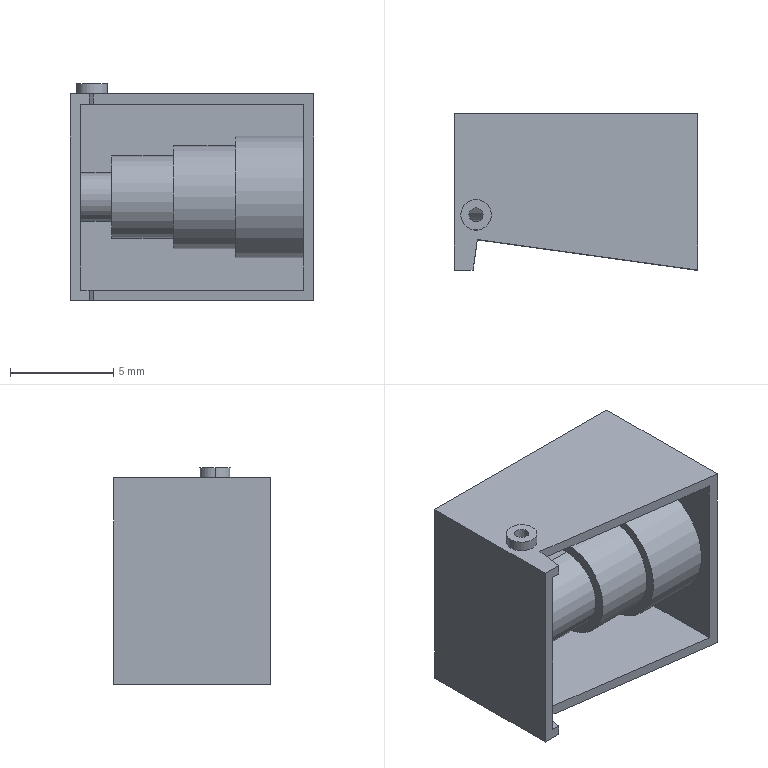Part | SolidWorks | features ICE 8, Extrusion 1, Shell 1 | 1 solid | 35 faces | box 11.794 x 7.578 x 10.5 mm | volume 389.974 mm3 | plane 19 | cylinder 16 | commonest cylinder face diameters 0.684 x4 1.479 x2 1.676 x2 2.353 x2 4 x2 5 x2
STEP:
#1=CARTESIAN_POINT('',(-33.114,-4.039,-2.056));
#2=VERTEX_POINT('',#1);
#3=CARTESIAN_POINT('',(-33.114,-4.039,-7.944));
#4=VERTEX_POINT('',#3);
#5=CARTESIAN_POINT('',(-33.114,-4.039,-5.));
#6=DIRECTION('',(-1.,0.,0.));
#7=DIRECTION('',(0.,0.,-1.));
#8=AXIS2_PLACEMENT_3D('',#5,#6,#7);
#9=CIRCLE('',#8,2.944);
#10=EDGE_CURVE('',#2,#4,#9,.T.);
#11=ORIENTED_EDGE('',*,*,#10,.T.);
#12=CARTESIAN_POINT('',(-36.407,-4.039,-7.944));
#13=VERTEX_POINT('',#12);
#14=CARTESIAN_POINT('',(-24.786,-4.039,-7.944));
#15=DIRECTION('',(-1.,0.,0.));
#16=VECTOR('',#15,1000.);
#17=LINE('',#14,#16);
#18=EDGE_CURVE('',#4,#13,#17,.T.);
#19=ORIENTED_EDGE('',*,*,#18,.T.);
#20=CARTESIAN_POINT('',(-36.407,-4.039,-2.056));
#21=VERTEX_POINT('',#20);
#22=CARTESIAN_POINT('',(-36.407,-4.039,-5.));
#23=DIRECTION('',(1.,0.,0.));
#24=DIRECTION('',(0.,0.,-1.));
#25=AXIS2_PLACEMENT_3D('',#22,#23,#24);
#26=CIRCLE('',#25,2.944);
#27=EDGE_CURVE('',#13,#21,#26,.T.);
#28=ORIENTED_EDGE('',*,*,#27,.T.);
#29=CARTESIAN_POINT('',(-24.786,-4.039,-2.056));
#30=DIRECTION('',(-1.,0.,0.));
#31=VECTOR('',#30,1000.);
#32=LINE('',#29,#31);
#33=EDGE_CURVE('',#2,#21,#32,.T.);
#34=ORIENTED_EDGE('',*,*,#33,.F.);
#35=EDGE_LOOP('',(#11,#19,#28,#34));
#36=FACE_OUTER_BOUND('',#35,.T.);
#37=CARTESIAN_POINT('',(-24.786,-4.039,-5.));
#38=DIRECTION('',(-1.,0.,0.));
#39=DIRECTION('',(0.,0.,1.));
#40=AXIS2_PLACEMENT_3D('',#37,#38,#39);
#41=CYLINDRICAL_SURFACE('',#40,2.944);
#42=ADVANCED_FACE('',(#36),#41,.T.);
#43=CARTESIAN_POINT('',(-36.407,-4.039,-7.5));
#44=VERTEX_POINT('',#43);
#45=CARTESIAN_POINT('',(-36.407,-4.039,-2.5));
#46=VERTEX_POINT('',#45);
#47=CARTESIAN_POINT('',(-36.407,-4.039,-5.));
#48=DIRECTION('',(1.,0.,0.));
#49=DIRECTION('',(0.,0.,-1.));
#50=AXIS2_PLACEMENT_3D('',#47,#48,#49);
#51=CIRCLE('',#50,2.5);
#52=EDGE_CURVE('',#44,#46,#51,.T.);
#53=ORIENTED_EDGE('',*,*,#52,.F.);
#54=CARTESIAN_POINT('',(-39.407,-4.039,-7.5));
#55=VERTEX_POINT('',#54);
#56=CARTESIAN_POINT('',(-36.407,-4.039,-7.5));
#57=DIRECTION('',(-1.,0.,0.));
#58=VECTOR('',#57,1000.);
#59=LINE('',#56,#58);
#60=EDGE_CURVE('',#44,#55,#59,.T.);
#61=ORIENTED_EDGE('',*,*,#60,.T.);
#62=CARTESIAN_POINT('',(-39.407,-4.039,-2.5));
#63=VERTEX_POINT('',#62);
#64=CARTESIAN_POINT('',(-39.407,-4.039,-5.));
#65=DIRECTION('',(1.,0.,0.));
#66=DIRECTION('',(0.,0.,-1.));
#67=AXIS2_PLACEMENT_3D('',#64,#65,#66);
#68=CIRCLE('',#67,2.5);
#69=EDGE_CURVE('',#55,#63,#68,.T.);
#70=ORIENTED_EDGE('',*,*,#69,.T.);
#71=CARTESIAN_POINT('',(-36.407,-4.039,-2.5));
#72=DIRECTION('',(-1.,0.,0.));
#73=VECTOR('',#72,1000.);
#74=LINE('',#71,#73);
#75=EDGE_CURVE('',#46,#63,#74,.T.);
#76=ORIENTED_EDGE('',*,*,#75,.F.);
#77=EDGE_LOOP('',(#53,#61,#70,#76));
#78=FACE_OUTER_BOUND('',#77,.T.);
#79=CARTESIAN_POINT('',(-36.407,-4.039,-5.));
#80=DIRECTION('',(-1.,0.,0.));
#81=DIRECTION('',(0.,0.,1.));
#82=AXIS2_PLACEMENT_3D('',#79,#80,#81);
#83=CYLINDRICAL_SURFACE('',#82,2.5);
#84=ADVANCED_FACE('',(#78),#83,.T.);
#85=CARTESIAN_POINT('',(-39.407,-4.039,-7.));
#86=VERTEX_POINT('',#85);
#87=CARTESIAN_POINT('',(-39.407,-4.039,-3.));
#88=VERTEX_POINT('',#87);
#89=CARTESIAN_POINT('',(-39.407,-4.039,-5.));
#90=DIRECTION('',(1.,0.,0.));
#91=DIRECTION('',(0.,0.,-1.));
#92=AXIS2_PLACEMENT_3D('',#89,#90,#91);
#93=CIRCLE('',#92,2.);
#94=EDGE_CURVE('',#86,#88,#93,.T.);
#95=ORIENTED_EDGE('',*,*,#94,.F.);
#96=CARTESIAN_POINT('',(-42.407,-4.039,-7.));
#97=VERTEX_POINT('',#96);
#98=CARTESIAN_POINT('',(-39.407,-4.039,-7.));
#99=DIRECTION('',(-1.,0.,0.));
#100=VECTOR('',#99,1000.);
#101=LINE('',#98,#100);
#102=EDGE_CURVE('',#86,#97,#101,.T.);
#103=ORIENTED_EDGE('',*,*,#102,.T.);
#104=CARTESIAN_POINT('',(-42.407,-4.039,-3.));
#105=VERTEX_POINT('',#104);
#106=CARTESIAN_POINT('',(-42.407,-4.039,-5.));
#107=DIRECTION('',(1.,0.,0.));
#108=DIRECTION('',(0.,0.,-1.));
#109=AXIS2_PLACEMENT_3D('',#106,#107,#108);
#110=CIRCLE('',#109,2.);
#111=EDGE_CURVE('',#97,#105,#110,.T.);
#112=ORIENTED_EDGE('',*,*,#111,.T.);
#113=CARTESIAN_POINT('',(-39.407,-4.039,-3.));
#114=DIRECTION('',(-1.,0.,0.));
#115=VECTOR('',#114,1000.);
#116=LINE('',#113,#115);
#117=EDGE_CURVE('',#88,#105,#116,.T.);
#118=ORIENTED_EDGE('',*,*,#117,.F.);
#119=EDGE_LOOP('',(#95,#103,#112,#118));
#120=FACE_OUTER_BOUND('',#119,.T.);
#121=CARTESIAN_POINT('',(-39.407,-4.039,-5.));
#122=DIRECTION('',(-1.,0.,0.));
#123=DIRECTION('',(0.,0.,1.));
#124=AXIS2_PLACEMENT_3D('',#121,#122,#123);
#125=CYLINDRICAL_SURFACE('',#124,2.);
#126=ADVANCED_FACE('',(#120),#125,.T.);
#127=CARTESIAN_POINT('',(-42.407,-4.039,-6.177));
#128=VERTEX_POINT('',#127);
#129=CARTESIAN_POINT('',(-42.407,-4.039,-3.823));
#130=VERTEX_POINT('',#129);
#131=CARTESIAN_POINT('',(-42.407,-4.039,-5.));
#132=DIRECTION('',(1.,0.,0.));
#133=DIRECTION('',(0.,0.,-1.));
#134=AXIS2_PLACEMENT_3D('',#131,#132,#133);
#135=CIRCLE('',#134,1.177);
#136=EDGE_CURVE('',#128,#130,#135,.T.);
#137=ORIENTED_EDGE('',*,*,#136,.F.);
#138=CARTESIAN_POINT('',(-43.907,-4.039,-6.177));
#139=VERTEX_POINT('',#138);
#140=CARTESIAN_POINT('',(-42.407,-4.039,-6.177));
#141=DIRECTION('',(-1.,0.,0.));
#142=VECTOR('',#141,1000.);
#143=LINE('',#140,#142);
#144=EDGE_CURVE('',#128,#139,#143,.T.);
#145=ORIENTED_EDGE('',*,*,#144,.T.);
#146=CARTESIAN_POINT('',(-43.907,-4.039,-3.823));
#147=VERTEX_POINT('',#146);
#148=CARTESIAN_POINT('',(-43.907,-4.039,-5.));
#149=DIRECTION('',(1.,0.,0.));
#150=DIRECTION('',(0.,0.,1.));
#151=AXIS2_PLACEMENT_3D('',#148,#149,#150);
#152=CIRCLE('',#151,1.177);
#153=EDGE_CURVE('',#139,#147,#152,.T.);
#154=ORIENTED_EDGE('',*,*,#153,.T.);
#155=CARTESIAN_POINT('',(-42.407,-4.039,-3.823));
#156=DIRECTION('',(-1.,0.,0.));
#157=VECTOR('',#156,1000.);
#158=LINE('',#155,#157);
#159=EDGE_CURVE('',#130,#147,#158,.T.);
#160=ORIENTED_EDGE('',*,*,#159,.F.);
#161=EDGE_LOOP('',(#137,#145,#154,#160));
#162=FACE_OUTER_BOUND('',#161,.T.);
#163=CARTESIAN_POINT('',(-42.407,-4.039,-5.));
#164=DIRECTION('',(-1.,0.,0.));
#165=DIRECTION('',(0.,0.,1.));
#166=AXIS2_PLACEMENT_3D('',#163,#164,#165);
#167=CYLINDRICAL_SURFACE('',#166,1.177);
#168=ADVANCED_FACE('',(#162),#167,.T.);
#169=CARTESIAN_POINT('',(-32.614,-3.789,-5.838));
#170=VERTEX_POINT('',#169);
#171=CARTESIAN_POINT('',(-32.614,-3.789,-4.162));
#172=VERTEX_POINT('',#171);
#173=CARTESIAN_POINT('',(-32.614,-3.789,-5.));
#174=DIRECTION('',(-1.,0.,0.));
#175=DIRECTION('',(0.,0.,-1.));
#176=AXIS2_PLACEMENT_3D('',#173,#174,#175);
#177=CIRCLE('',#176,0.8381);
#178=EDGE_CURVE('',#170,#172,#177,.T.);
#179=ORIENTED_EDGE('',*,*,#178,.F.);
#180=CARTESIAN_POINT('',(-33.114,-3.789,-5.838));
#181=VERTEX_POINT('',#180);
#182=CARTESIAN_POINT('',(-32.614,-3.789,-5.838));
#183=DIRECTION('',(-1.,0.,0.));
#184=VECTOR('',#183,1000.);
#185=LINE('',#182,#184);
#186=EDGE_CURVE('',#170,#181,#185,.T.);
#187=ORIENTED_EDGE('',*,*,#186,.T.);
#188=CARTESIAN_POINT('',(-33.114,-3.789,-4.162));
#189=VERTEX_POINT('',#188);
#190=CARTESIAN_POINT('',(-33.114,-3.789,-5.));
#191=DIRECTION('',(1.,0.,0.));
#192=DIRECTION('',(0.,0.,-1.));
#193=AXIS2_PLACEMENT_3D('',#190,#191,#192);
#194=CIRCLE('',#193,0.8381);
#195=EDGE_CURVE('',#189,#181,#194,.T.);
#196=ORIENTED_EDGE('',*,*,#195,.F.);
#197=CARTESIAN_POINT('',(-32.614,-3.789,-4.162));
#198=DIRECTION('',(-1.,0.,0.));
#199=VECTOR('',#198,1000.);
#200=LINE('',#197,#199);
#201=EDGE_CURVE('',#172,#189,#200,.T.);
#202=ORIENTED_EDGE('',*,*,#201,.F.);
#203=EDGE_LOOP('',(#179,#187,#196,#202));
#204=FACE_OUTER_BOUND('',#203,.T.);
#205=CARTESIAN_POINT('',(-32.614,-3.789,-5.));
#206=DIRECTION('',(-1.,0.,0.));
#207=DIRECTION('',(0.,0.,1.));
#208=AXIS2_PLACEMENT_3D('',#205,#206,#207);
#209=CYLINDRICAL_SURFACE('',#208,0.8381);
#210=ADVANCED_FACE('',(#204),#209,.F.);
#211=CARTESIAN_POINT('',(-43.691,-4.904,-10.));
#212=VERTEX_POINT('',#211);
#213=CARTESIAN_POINT('',(-43.007,-4.904,-10.));
#214=VERTEX_POINT('',#213);
#215=CARTESIAN_POINT('',(-43.349,-4.904,-10.));
#216=DIRECTION('',(0.,0.,1.));
#217=DIRECTION('',(1.,0.,0.));
#218=AXIS2_PLACEMENT_3D('',#215,#216,#217);
#219=CIRCLE('',#218,0.3422);
#220=EDGE_CURVE('',#212,#214,#219,.T.);
#221=ORIENTED_EDGE('',*,*,#220,.F.);
#222=CARTESIAN_POINT('',(-43.691,-4.904,-9.5));
#223=VERTEX_POINT('',#222);
#224=CARTESIAN_POINT('',(-43.691,-4.904,-10.));
#225=DIRECTION('',(0.,0.,1.));
#226=VECTOR('',#225,1000.);
#227=LINE('',#224,#226);
#228=EDGE_CURVE('',#212,#223,#227,.T.);
#229=ORIENTED_EDGE('',*,*,#228,.T.);
#230=CARTESIAN_POINT('',(-43.007,-4.904,-9.5));
#231=VERTEX_POINT('',#230);
#232=CARTESIAN_POINT('',(-43.349,-4.904,-9.5));
#233=DIRECTION('',(0.,0.,1.));
#234=DIRECTION('',(1.,0.,0.));
#235=AXIS2_PLACEMENT_3D('',#232,#233,#234);
#236=CIRCLE('',#235,0.3422);
#237=EDGE_CURVE('',#223,#231,#236,.T.);
#238=ORIENTED_EDGE('',*,*,#237,.T.);
#239=CARTESIAN_POINT('',(-43.007,-4.904,-10.));
#240=DIRECTION('',(0.,0.,1.));
#241=VECTOR('',#240,1000.);
#242=LINE('',#239,#241);
#243=EDGE_CURVE('',#214,#231,#242,.T.);
#244=ORIENTED_EDGE('',*,*,#243,.F.);
#245=EDGE_LOOP('',(#221,#229,#238,#244));
#246=FACE_OUTER_BOUND('',#245,.T.);
#247=CARTESIAN_POINT('',(-43.349,-4.904,-10.));
#248=DIRECTION('',(0.,0.,1.));
#249=DIRECTION('',(1.,0.,0.));
#250=AXIS2_PLACEMENT_3D('',#247,#248,#249);
#251=CYLINDRICAL_SURFACE('',#250,0.3422);
#252=ADVANCED_FACE('',(#246),#251,.F.);
#253=CARTESIAN_POINT('',(-43.007,-4.904,-0.5));
#254=VERTEX_POINT('',#253);
#255=CARTESIAN_POINT('',(-43.691,-4.904,-0.5));
#256=VERTEX_POINT('',#255);
#257=CARTESIAN_POINT('',(-43.349,-4.904,-0.5));
#258=DIRECTION('',(0.,0.,-1.));
#259=DIRECTION('',(-1.,0.,0.));
#260=AXIS2_PLACEMENT_3D('',#257,#258,#259);
#261=CIRCLE('',#260,0.3422);
#262=EDGE_CURVE('',#254,#256,#261,.T.);
#263=ORIENTED_EDGE('',*,*,#262,.T.);
#264=CARTESIAN_POINT('',(-43.691,-4.904,0.5));
#265=VERTEX_POINT('',#264);
#266=CARTESIAN_POINT('',(-43.691,-4.904,-10.));
#267=DIRECTION('',(0.,0.,1.));
#268=VECTOR('',#267,1000.);
#269=LINE('',#266,#268);
#270=EDGE_CURVE('',#256,#265,#269,.T.);
#271=ORIENTED_EDGE('',*,*,#270,.T.);
#272=CARTESIAN_POINT('',(-43.007,-4.904,0.5));
#273=VERTEX_POINT('',#272);
#274=CARTESIAN_POINT('',(-43.349,-4.904,0.5));
#275=DIRECTION('',(0.,0.,1.));
#276=DIRECTION('',(1.,0.,0.));
#277=AXIS2_PLACEMENT_3D('',#274,#275,#276);
#278=CIRCLE('',#277,0.3422);
#279=EDGE_CURVE('',#265,#273,#278,.T.);
#280=ORIENTED_EDGE('',*,*,#279,.T.);
#281=CARTESIAN_POINT('',(-43.007,-4.904,-10.));
#282=DIRECTION('',(0.,0.,1.));
#283=VECTOR('',#282,1000.);
#284=LINE('',#281,#283);
#285=EDGE_CURVE('',#254,#273,#284,.T.);
#286=ORIENTED_EDGE('',*,*,#285,.F.);
#287=EDGE_LOOP('',(#263,#271,#280,#286));
#288=FACE_OUTER_BOUND('',#287,.T.);
#289=CARTESIAN_POINT('',(-43.349,-4.904,-10.));
#290=DIRECTION('',(0.,0.,1.));
#291=DIRECTION('',(1.,0.,0.));
#292=AXIS2_PLACEMENT_3D('',#289,#290,#291);
#293=CYLINDRICAL_SURFACE('',#292,0.3422);
#294=ADVANCED_FACE('',(#288),#293,.F.);
#295=CARTESIAN_POINT('',(-42.609,-4.904,0.5));
#296=VERTEX_POINT('',#295);
#297=CARTESIAN_POINT('',(-44.088,-4.904,0.5));
#298=VERTEX_POINT('',#297);
#299=CARTESIAN_POINT('',(-43.349,-4.904,0.5));
#300=DIRECTION('',(0.,0.,1.));
#301=DIRECTION('',(1.,0.,0.));
#302=AXIS2_PLACEMENT_3D('',#299,#300,#301);
#303=CIRCLE('',#302,0.7394);
#304=EDGE_CURVE('',#296,#298,#303,.T.);
#305=ORIENTED_EDGE('',*,*,#304,.F.);
#306=CARTESIAN_POINT('',(-42.609,-4.904,0.));
#307=VERTEX_POINT('',#306);
#308=CARTESIAN_POINT('',(-42.609,-4.904,0.5));
#309=DIRECTION('',(0.,0.,-1.));
#310=VECTOR('',#309,1000.);
#311=LINE('',#308,#310);
#312=EDGE_CURVE('',#296,#307,#311,.T.);
#313=ORIENTED_EDGE('',*,*,#312,.T.);
#314=CARTESIAN_POINT('',(-44.088,-4.904,0.));
#315=VERTEX_POINT('',#314);
#316=CARTESIAN_POINT('',(-43.349,-4.904,0.));
#317=DIRECTION('',(0.,0.,1.));
#318=DIRECTION('',(-1.,0.,0.));
#319=AXIS2_PLACEMENT_3D('',#316,#317,#318);
#320=CIRCLE('',#319,0.7394);
#321=EDGE_CURVE('',#307,#315,#320,.T.);
#322=ORIENTED_EDGE('',*,*,#321,.T.);
#323=CARTESIAN_POINT('',(-44.088,-4.904,0.5));
#324=DIRECTION('',(0.,0.,-1.));
#325=VECTOR('',#324,1000.);
#326=LINE('',#323,#325);
#327=EDGE_CURVE('',#298,#315,#326,.T.);
#328=ORIENTED_EDGE('',*,*,#327,.F.);
#329=EDGE_LOOP('',(#305,#313,#322,#328));
#330=FACE_OUTER_BOUND('',#329,.T.);
#331=CARTESIAN_POINT('',(-43.349,-4.904,0.5));
#332=DIRECTION('',(0.,0.,-1.));
#333=DIRECTION('',(-1.,0.,0.));
#334=AXIS2_PLACEMENT_3D('',#331,#332,#333);
#335=CYLINDRICAL_SURFACE('',#334,0.7394);
#336=ADVANCED_FACE('',(#330),#335,.T.);
#337=CARTESIAN_POINT('',(-43.493,-7.578,-0.5));
#338=VERTEX_POINT('',#337);
#339=CARTESIAN_POINT('',(-43.493,-7.578,0.));
#340=VERTEX_POINT('',#339);
#341=CARTESIAN_POINT('',(-43.493,-7.578,-10.));
#342=DIRECTION('',(0.,0.,1.));
#343=VECTOR('',#342,1000.);
#344=LINE('',#341,#343);
#345=EDGE_CURVE('',#338,#340,#344,.T.);
#346=ORIENTED_EDGE('',*,*,#345,.T.);
#347=CARTESIAN_POINT('',(-44.407,-7.578,0.));
#348=VERTEX_POINT('',#347);
#349=CARTESIAN_POINT('',(-32.614,-7.578,0.));
#350=DIRECTION('',(1.,0.,0.));
#351=VECTOR('',#350,1000.);
#352=LINE('',#349,#351);
#353=EDGE_CURVE('',#348,#340,#352,.T.);
#354=ORIENTED_EDGE('',*,*,#353,.F.);
#355=CARTESIAN_POINT('',(-44.407,-7.578,-10.));
#356=VERTEX_POINT('',#355);
#357=CARTESIAN_POINT('',(-44.407,-7.578,-24.018));
#358=DIRECTION('',(0.,0.,1.));
#359=VECTOR('',#358,1000.);
#360=LINE('',#357,#359);
#361=EDGE_CURVE('',#356,#348,#360,.T.);
#362=ORIENTED_EDGE('',*,*,#361,.F.);
#363=CARTESIAN_POINT('',(-43.493,-7.578,-10.));
#364=VERTEX_POINT('',#363);
#365=CARTESIAN_POINT('',(-32.614,-7.578,-10.));
#366=DIRECTION('',(-1.,0.,0.));
#367=VECTOR('',#366,1000.);
#368=LINE('',#365,#367);
#369=EDGE_CURVE('',#364,#356,#368,.T.);
#370=ORIENTED_EDGE('',*,*,#369,.F.);
#371=CARTESIAN_POINT('',(-43.493,-7.578,-9.5));
#372=VERTEX_POINT('',#371);
#373=CARTESIAN_POINT('',(-43.493,-7.578,-10.));
#374=DIRECTION('',(0.,0.,1.));
#375=VECTOR('',#374,1000.);
#376=LINE('',#373,#375);
#377=EDGE_CURVE('',#364,#372,#376,.T.);
#378=ORIENTED_EDGE('',*,*,#377,.T.);
#379=CARTESIAN_POINT('',(-43.907,-7.578,-9.5));
#380=VERTEX_POINT('',#379);
#381=CARTESIAN_POINT('',(-32.614,-7.578,-9.5));
#382=DIRECTION('',(-1.,0.,0.));
#383=VECTOR('',#382,1000.);
#384=LINE('',#381,#383);
#385=EDGE_CURVE('',#372,#380,#384,.T.);
#386=ORIENTED_EDGE('',*,*,#385,.T.);
#387=CARTESIAN_POINT('',(-43.907,-7.578,-0.5));
#388=VERTEX_POINT('',#387);
#389=CARTESIAN_POINT('',(-43.907,-7.578,-24.018));
#390=DIRECTION('',(0.,0.,1.));
#391=VECTOR('',#390,1000.);
#392=LINE('',#389,#391);
#393=EDGE_CURVE('',#380,#388,#392,.T.);
#394=ORIENTED_EDGE('',*,*,#393,.T.);
#395=CARTESIAN_POINT('',(-32.614,-7.578,-0.5));
#396=DIRECTION('',(1.,0.,0.));
#397=VECTOR('',#396,1000.);
#398=LINE('',#395,#397);
#399=EDGE_CURVE('',#388,#338,#398,.T.);
#400=ORIENTED_EDGE('',*,*,#399,.T.);
#401=EDGE_LOOP('',(#346,#354,#362,#370,#378,#386,#394,#400));
#402=FACE_OUTER_BOUND('',#401,.T.);
#403=CARTESIAN_POINT('',(-32.614,-7.578,-24.018));
#404=DIRECTION('',(0.,-1.,0.));
#405=DIRECTION('',(0.,0.,-1.));
#406=AXIS2_PLACEMENT_3D('',#403,#404,#405);
#407=PLANE('',#406);
#408=ADVANCED_FACE('',(#402),#407,.T.);
#409=CARTESIAN_POINT('',(-32.614,-3.789,-5.));
#410=DIRECTION('',(-1.,0.,0.));
#411=DIRECTION('',(0.,0.,-1.));
#412=AXIS2_PLACEMENT_3D('',#409,#410,#411);
#413=CIRCLE('',#412,0.8381);
#414=EDGE_CURVE('',#172,#170,#413,.T.);
#415=ORIENTED_EDGE('',*,*,#414,.T.);
#416=ORIENTED_EDGE('',*,*,#178,.T.);
#417=EDGE_LOOP('',(#415,#416));
#418=FACE_BOUND('',#417,.T.);
#419=CARTESIAN_POINT('',(-32.614,0.,-10.));
#420=VERTEX_POINT('',#419);
#421=CARTESIAN_POINT('',(-32.614,-7.578,-10.));
#422=VERTEX_POINT('',#421);
#423=CARTESIAN_POINT('',(-32.614,0.,-10.));
#424=DIRECTION('',(0.,-1.,0.));
#425=VECTOR('',#424,1000.);
#426=LINE('',#423,#425);
#427=EDGE_CURVE('',#420,#422,#426,.T.);
#428=ORIENTED_EDGE('',*,*,#427,.F.);
#429=CARTESIAN_POINT('',(-32.614,0.,0.));
#430=VERTEX_POINT('',#429);
#431=CARTESIAN_POINT('',(-32.614,0.,-24.018));
#432=DIRECTION('',(0.,0.,1.));
#433=VECTOR('',#432,1000.);
#434=LINE('',#431,#433);
#435=EDGE_CURVE('',#420,#430,#434,.T.);
#436=ORIENTED_EDGE('',*,*,#435,.T.);
#437=CARTESIAN_POINT('',(-32.614,-7.578,0.));
#438=VERTEX_POINT('',#437);
#439=CARTESIAN_POINT('',(-32.614,0.,0.));
#440=DIRECTION('',(0.,1.,0.));
#441=VECTOR('',#440,1000.);
#442=LINE('',#439,#441);
#443=EDGE_CURVE('',#438,#430,#442,.T.);
#444=ORIENTED_EDGE('',*,*,#443,.F.);
#445=CARTESIAN_POINT('',(-32.614,-7.578,-24.018));
#446=DIRECTION('',(0.,0.,1.));
#447=VECTOR('',#446,1000.);
#448=LINE('',#445,#447);
#449=EDGE_CURVE('',#422,#438,#448,.T.);
#450=ORIENTED_EDGE('',*,*,#449,.F.);
#451=EDGE_LOOP('',(#428,#436,#444,#450));
#452=FACE_OUTER_BOUND('',#451,.T.);
#453=CARTESIAN_POINT('',(-32.614,0.,-24.018));
#454=DIRECTION('',(1.,0.,0.));
#455=DIRECTION('',(0.,0.,-1.));
#456=AXIS2_PLACEMENT_3D('',#453,#454,#455);
#457=PLANE('',#456);
#458=ADVANCED_FACE('',(#418,#452),#457,.T.);
#459=CARTESIAN_POINT('',(-44.407,0.,-10.));
#460=VERTEX_POINT('',#459);
#461=CARTESIAN_POINT('',(-44.407,0.,-10.));
#462=DIRECTION('',(0.,1.,0.));
#463=VECTOR('',#462,1000.);
#464=LINE('',#461,#463);
#465=EDGE_CURVE('',#356,#460,#464,.T.);
#466=ORIENTED_EDGE('',*,*,#465,.F.);
#467=ORIENTED_EDGE('',*,*,#361,.T.);
#468=CARTESIAN_POINT('',(-44.407,0.,0.));
#469=VERTEX_POINT('',#468);
#470=CARTESIAN_POINT('',(-44.407,0.,0.));
#471=DIRECTION('',(0.,-1.,0.));
#472=VECTOR('',#471,1000.);
#473=LINE('',#470,#472);
#474=EDGE_CURVE('',#469,#348,#473,.T.);
#475=ORIENTED_EDGE('',*,*,#474,.F.);
#476=CARTESIAN_POINT('',(-44.407,0.,-24.018));
#477=DIRECTION('',(0.,0.,1.));
#478=VECTOR('',#477,1000.);
#479=LINE('',#476,#478);
#480=EDGE_CURVE('',#460,#469,#479,.T.);
#481=ORIENTED_EDGE('',*,*,#480,.F.);
#482=EDGE_LOOP('',(#466,#467,#475,#481));
#483=FACE_OUTER_BOUND('',#482,.T.);
#484=CARTESIAN_POINT('',(-44.407,0.,-24.018));
#485=DIRECTION('',(-1.,0.,0.));
#486=DIRECTION('',(0.,0.,1.));
#487=AXIS2_PLACEMENT_3D('',#484,#485,#486);
#488=PLANE('',#487);
#489=ADVANCED_FACE('',(#483),#488,.T.);
#490=CARTESIAN_POINT('',(-32.614,0.,-10.));
#491=DIRECTION('',(1.,0.,0.));
#492=VECTOR('',#491,1000.);
#493=LINE('',#490,#492);
#494=EDGE_CURVE('',#460,#420,#493,.T.);
#495=ORIENTED_EDGE('',*,*,#494,.F.);
#496=ORIENTED_EDGE('',*,*,#480,.T.);
#497=CARTESIAN_POINT('',(-32.614,0.,0.));
#498=DIRECTION('',(-1.,0.,0.));
#499=VECTOR('',#498,1000.);
#500=LINE('',#497,#499);
#501=EDGE_CURVE('',#430,#469,#500,.T.);
#502=ORIENTED_EDGE('',*,*,#501,.F.);
#503=ORIENTED_EDGE('',*,*,#435,.F.);
#504=EDGE_LOOP('',(#495,#496,#502,#503));
#505=FACE_OUTER_BOUND('',#504,.T.);
#506=CARTESIAN_POINT('',(-32.614,0.,-24.018));
#507=DIRECTION('',(0.,1.,0.));
#508=DIRECTION('',(0.,0.,1.));
#509=AXIS2_PLACEMENT_3D('',#506,#507,#508);
#510=PLANE('',#509);
#511=ADVANCED_FACE('',(#505),#510,.T.);
#512=CARTESIAN_POINT('',(-43.349,-4.904,0.));
#513=DIRECTION('',(0.,0.,1.));
#514=DIRECTION('',(-1.,0.,0.));
#515=AXIS2_PLACEMENT_3D('',#512,#513,#514);
#516=CIRCLE('',#515,0.7394);
#517=EDGE_CURVE('',#315,#307,#516,.T.);
#518=ORIENTED_EDGE('',*,*,#517,.F.);
#519=ORIENTED_EDGE('',*,*,#321,.F.);
#520=EDGE_LOOP('',(#518,#519));
#521=FACE_BOUND('',#520,.T.);
#522=ORIENTED_EDGE('',*,*,#353,.T.);
#523=CARTESIAN_POINT('',(-43.288,-6.099,0.));
#524=VERTEX_POINT('',#523);
#525=CARTESIAN_POINT('',(-41.643,5.77,0.));
#526=DIRECTION('',(0.1373,0.9905,0.));
#527=VECTOR('',#526,1000.);
#528=LINE('',#525,#527);
#529=EDGE_CURVE('',#340,#524,#528,.T.);
#530=ORIENTED_EDGE('',*,*,#529,.T.);
#531=CARTESIAN_POINT('',(-1.645,-11.869,0.));
#532=DIRECTION('',(0.9905,-0.1373,0.));
#533=VECTOR('',#532,1000.);
#534=LINE('',#531,#533);
#535=EDGE_CURVE('',#524,#438,#534,.T.);
#536=ORIENTED_EDGE('',*,*,#535,.T.);
#537=ORIENTED_EDGE('',*,*,#443,.T.);
#538=ORIENTED_EDGE('',*,*,#501,.T.);
#539=ORIENTED_EDGE('',*,*,#474,.T.);
#540=EDGE_LOOP('',(#522,#530,#536,#537,#538,#539));
#541=FACE_OUTER_BOUND('',#540,.T.);
#542=CARTESIAN_POINT('',(0.,0.,0.));
#543=DIRECTION('',(0.,0.,-1.));
#544=DIRECTION('',(-1.,0.,0.));
#545=AXIS2_PLACEMENT_3D('',#542,#543,#544);
#546=PLANE('',#545);
#547=ADVANCED_FACE('',(#521,#541),#546,.F.);
#548=CARTESIAN_POINT('',(-43.349,-4.904,-10.));
#549=DIRECTION('',(0.,0.,1.));
#550=DIRECTION('',(1.,0.,0.));
#551=AXIS2_PLACEMENT_3D('',#548,#549,#550);
#552=CIRCLE('',#551,0.3422);
#553=EDGE_CURVE('',#214,#212,#552,.T.);
#554=ORIENTED_EDGE('',*,*,#553,.T.);
#555=ORIENTED_EDGE('',*,*,#220,.T.);
#556=EDGE_LOOP('',(#554,#555));
#557=FACE_BOUND('',#556,.T.);
#558=CARTESIAN_POINT('',(-43.288,-6.099,-10.));
#559=VERTEX_POINT('',#558);
#560=CARTESIAN_POINT('',(-32.614,-7.578,-10.));
#561=DIRECTION('',(-0.9905,0.1373,0.));
#562=VECTOR('',#561,1000.);
#563=LINE('',#560,#562);
#564=EDGE_CURVE('',#422,#559,#563,.T.);
#565=ORIENTED_EDGE('',*,*,#564,.T.);
#566=CARTESIAN_POINT('',(-43.288,-6.099,-10.));
#567=DIRECTION('',(-0.1373,-0.9905,0.));
#568=VECTOR('',#567,1000.);
#569=LINE('',#566,#568);
#570=EDGE_CURVE('',#559,#364,#569,.T.);
#571=ORIENTED_EDGE('',*,*,#570,.T.);
#572=ORIENTED_EDGE('',*,*,#369,.T.);
#573=ORIENTED_EDGE('',*,*,#465,.T.);
#574=ORIENTED_EDGE('',*,*,#494,.T.);
#575=ORIENTED_EDGE('',*,*,#427,.T.);
#576=EDGE_LOOP('',(#565,#571,#572,#573,#574,#575));
#577=FACE_OUTER_BOUND('',#576,.T.);
#578=CARTESIAN_POINT('',(0.,20.,-10.));
#579=DIRECTION('',(0.,0.,1.));
#580=DIRECTION('',(1.,0.,0.));
#581=AXIS2_PLACEMENT_3D('',#578,#579,#580);
#582=PLANE('',#581);
#583=ADVANCED_FACE('',(#557,#577),#582,.F.);
#584=ORIENTED_EDGE('',*,*,#10,.F.);
#585=CARTESIAN_POINT('',(-33.114,-4.039,-5.));
#586=DIRECTION('',(-1.,0.,0.));
#587=DIRECTION('',(0.,0.,-1.));
#588=AXIS2_PLACEMENT_3D('',#585,#586,#587);
#589=CIRCLE('',#588,2.944);
#590=EDGE_CURVE('',#4,#2,#589,.T.);
#591=ORIENTED_EDGE('',*,*,#590,.F.);
#592=EDGE_LOOP('',(#584,#591));
#593=FACE_BOUND('',#592,.T.);
#594=CARTESIAN_POINT('',(-33.114,-0.5,-9.5));
#595=VERTEX_POINT('',#594);
#596=CARTESIAN_POINT('',(-33.114,-7.508,-9.5));
#597=VERTEX_POINT('',#596);
#598=CARTESIAN_POINT('',(-33.114,0.,-9.5));
#599=DIRECTION('',(0.,-1.,0.));
#600=VECTOR('',#599,1000.);
#601=LINE('',#598,#600);
#602=EDGE_CURVE('',#595,#597,#601,.T.);
#603=ORIENTED_EDGE('',*,*,#602,.T.);
#604=CARTESIAN_POINT('',(-33.114,-7.508,-0.5));
#605=VERTEX_POINT('',#604);
#606=CARTESIAN_POINT('',(-33.114,-7.508,-24.018));
#607=DIRECTION('',(0.,0.,1.));
#608=VECTOR('',#607,1000.);
#609=LINE('',#606,#608);
#610=EDGE_CURVE('',#597,#605,#609,.T.);
#611=ORIENTED_EDGE('',*,*,#610,.T.);
#612=CARTESIAN_POINT('',(-33.114,-0.5,-0.5));
#613=VERTEX_POINT('',#612);
#614=CARTESIAN_POINT('',(-33.114,0.,-0.5));
#615=DIRECTION('',(0.,1.,0.));
#616=VECTOR('',#615,1000.);
#617=LINE('',#614,#616);
#618=EDGE_CURVE('',#605,#613,#617,.T.);
#619=ORIENTED_EDGE('',*,*,#618,.T.);
#620=CARTESIAN_POINT('',(-33.114,-0.5,-24.018));
#621=DIRECTION('',(0.,0.,1.));
#622=VECTOR('',#621,1000.);
#623=LINE('',#620,#622);
#624=EDGE_CURVE('',#595,#613,#623,.T.);
#625=ORIENTED_EDGE('',*,*,#624,.F.);
#626=EDGE_LOOP('',(#603,#611,#619,#625));
#627=FACE_OUTER_BOUND('',#626,.T.);
#628=CARTESIAN_POINT('',(-33.114,0.,-24.018));
#629=DIRECTION('',(1.,0.,0.));
#630=DIRECTION('',(0.,0.,-1.));
#631=AXIS2_PLACEMENT_3D('',#628,#629,#630);
#632=PLANE('',#631);
#633=ADVANCED_FACE('',(#593,#627),#632,.F.);
#634=CARTESIAN_POINT('',(-43.907,-4.039,-5.));
#635=DIRECTION('',(1.,0.,0.));
#636=DIRECTION('',(0.,0.,1.));
#637=AXIS2_PLACEMENT_3D('',#634,#635,#636);
#638=CIRCLE('',#637,1.177);
#639=EDGE_CURVE('',#147,#139,#638,.T.);
#640=ORIENTED_EDGE('',*,*,#639,.F.);
#641=ORIENTED_EDGE('',*,*,#153,.F.);
#642=EDGE_LOOP('',(#640,#641));
#643=FACE_BOUND('',#642,.T.);
#644=CARTESIAN_POINT('',(-43.907,-0.5,-9.5));
#645=VERTEX_POINT('',#644);
#646=CARTESIAN_POINT('',(-43.907,0.,-9.5));
#647=DIRECTION('',(0.,1.,0.));
#648=VECTOR('',#647,1000.);
#649=LINE('',#646,#648);
#650=EDGE_CURVE('',#380,#645,#649,.T.);
#651=ORIENTED_EDGE('',*,*,#650,.T.);
#652=CARTESIAN_POINT('',(-43.907,-0.5,-0.5));
#653=VERTEX_POINT('',#652);
#654=CARTESIAN_POINT('',(-43.907,-0.5,-24.018));
#655=DIRECTION('',(0.,0.,1.));
#656=VECTOR('',#655,1000.);
#657=LINE('',#654,#656);
#658=EDGE_CURVE('',#645,#653,#657,.T.);
#659=ORIENTED_EDGE('',*,*,#658,.T.);
#660=CARTESIAN_POINT('',(-43.907,0.,-0.5));
#661=DIRECTION('',(0.,-1.,0.));
#662=VECTOR('',#661,1000.);
#663=LINE('',#660,#662);
#664=EDGE_CURVE('',#653,#388,#663,.T.);
#665=ORIENTED_EDGE('',*,*,#664,.T.);
#666=ORIENTED_EDGE('',*,*,#393,.F.);
#667=EDGE_LOOP('',(#651,#659,#665,#666));
#668=FACE_OUTER_BOUND('',#667,.T.);
#669=CARTESIAN_POINT('',(-43.907,0.,-24.018));
#670=DIRECTION('',(-1.,0.,0.));
#671=DIRECTION('',(0.,0.,1.));
#672=AXIS2_PLACEMENT_3D('',#669,#670,#671);
#673=PLANE('',#672);
#674=ADVANCED_FACE('',(#643,#668),#673,.F.);
#675=CARTESIAN_POINT('',(-32.614,-0.5,-9.5));
#676=DIRECTION('',(1.,0.,0.));
#677=VECTOR('',#676,1000.);
#678=LINE('',#675,#677);
#679=EDGE_CURVE('',#645,#595,#678,.T.);
#680=ORIENTED_EDGE('',*,*,#679,.T.);
#681=ORIENTED_EDGE('',*,*,#624,.T.);
#682=CARTESIAN_POINT('',(-32.614,-0.5,-0.5));
#683=DIRECTION('',(-1.,0.,0.));
#684=VECTOR('',#683,1000.);
#685=LINE('',#682,#684);
#686=EDGE_CURVE('',#613,#653,#685,.T.);
#687=ORIENTED_EDGE('',*,*,#686,.T.);
#688=ORIENTED_EDGE('',*,*,#658,.F.);
#689=EDGE_LOOP('',(#680,#681,#687,#688));
#690=FACE_OUTER_BOUND('',#689,.T.);
#691=CARTESIAN_POINT('',(-32.614,-0.5,-24.018));
#692=DIRECTION('',(0.,1.,0.));
#693=DIRECTION('',(0.,0.,1.));
#694=AXIS2_PLACEMENT_3D('',#691,#692,#693);
#695=PLANE('',#694);
#696=ADVANCED_FACE('',(#690),#695,.F.);
#697=ORIENTED_EDGE('',*,*,#262,.F.);
#698=CARTESIAN_POINT('',(-43.349,-4.904,-0.5));
#699=DIRECTION('',(0.,0.,-1.));
#700=DIRECTION('',(-1.,0.,0.));
#701=AXIS2_PLACEMENT_3D('',#698,#699,#700);
#702=CIRCLE('',#701,0.3422);
#703=EDGE_CURVE('',#256,#254,#702,.T.);
#704=ORIENTED_EDGE('',*,*,#703,.F.);
#705=EDGE_LOOP('',(#697,#704));
#706=FACE_BOUND('',#705,.T.);
#707=CARTESIAN_POINT('',(-43.288,-6.099,-0.5));
#708=VERTEX_POINT('',#707);
#709=CARTESIAN_POINT('',(-41.643,5.77,-0.5));
#710=DIRECTION('',(0.1373,0.9905,0.));
#711=VECTOR('',#710,1000.);
#712=LINE('',#709,#711);
#713=EDGE_CURVE('',#338,#708,#712,.T.);
#714=ORIENTED_EDGE('',*,*,#713,.F.);
#715=ORIENTED_EDGE('',*,*,#399,.F.);
#716=ORIENTED_EDGE('',*,*,#664,.F.);
#717=ORIENTED_EDGE('',*,*,#686,.F.);
#718=ORIENTED_EDGE('',*,*,#618,.F.);
#719=CARTESIAN_POINT('',(-1.645,-11.869,-0.5));
#720=DIRECTION('',(0.9905,-0.1373,0.));
#721=VECTOR('',#720,1000.);
#722=LINE('',#719,#721);
#723=EDGE_CURVE('',#708,#605,#722,.T.);
#724=ORIENTED_EDGE('',*,*,#723,.F.);
#725=EDGE_LOOP('',(#714,#715,#716,#717,#718,#724));
#726=FACE_OUTER_BOUND('',#725,.T.);
#727=CARTESIAN_POINT('',(0.,0.,-0.5));
#728=DIRECTION('',(0.,0.,-1.));
#729=DIRECTION('',(-1.,0.,0.));
#730=AXIS2_PLACEMENT_3D('',#727,#728,#729);
#731=PLANE('',#730);
#732=ADVANCED_FACE('',(#706,#726),#731,.T.);
#733=CARTESIAN_POINT('',(-43.349,-4.904,-9.5));
#734=DIRECTION('',(0.,0.,1.));
#735=DIRECTION('',(1.,0.,0.));
#736=AXIS2_PLACEMENT_3D('',#733,#734,#735);
#737=CIRCLE('',#736,0.3422);
#738=EDGE_CURVE('',#231,#223,#737,.T.);
#739=ORIENTED_EDGE('',*,*,#738,.F.);
#740=ORIENTED_EDGE('',*,*,#237,.F.);
#741=EDGE_LOOP('',(#739,#740));
#742=FACE_BOUND('',#741,.T.);
#743=CARTESIAN_POINT('',(-43.288,-6.099,-9.5));
#744=VERTEX_POINT('',#743);
#745=CARTESIAN_POINT('',(-38.924,25.393,-9.5));
#746=DIRECTION('',(-0.1373,-0.9905,0.));
#747=VECTOR('',#746,1000.);
#748=LINE('',#745,#747);
#749=EDGE_CURVE('',#744,#372,#748,.T.);
#750=ORIENTED_EDGE('',*,*,#749,.F.);
#751=CARTESIAN_POINT('',(-4.364,-11.492,-9.5));
#752=DIRECTION('',(-0.9905,0.1373,0.));
#753=VECTOR('',#752,1000.);
#754=LINE('',#751,#753);
#755=EDGE_CURVE('',#597,#744,#754,.T.);
#756=ORIENTED_EDGE('',*,*,#755,.F.);
#757=ORIENTED_EDGE('',*,*,#602,.F.);
#758=ORIENTED_EDGE('',*,*,#679,.F.);
#759=ORIENTED_EDGE('',*,*,#650,.F.);
#760=ORIENTED_EDGE('',*,*,#385,.F.);
#761=EDGE_LOOP('',(#750,#756,#757,#758,#759,#760));
#762=FACE_OUTER_BOUND('',#761,.T.);
#763=CARTESIAN_POINT('',(0.,20.,-9.5));
#764=DIRECTION('',(0.,0.,1.));
#765=DIRECTION('',(1.,0.,0.));
#766=AXIS2_PLACEMENT_3D('',#763,#764,#765);
#767=PLANE('',#766);
#768=ADVANCED_FACE('',(#742,#762),#767,.T.);
#769=ORIENTED_EDGE('',*,*,#345,.F.);
#770=ORIENTED_EDGE('',*,*,#713,.T.);
#771=CARTESIAN_POINT('',(-43.288,-6.099,-10.));
#772=DIRECTION('',(0.,0.,1.));
#773=VECTOR('',#772,1000.);
#774=LINE('',#771,#773);
#775=EDGE_CURVE('',#708,#524,#774,.T.);
#776=ORIENTED_EDGE('',*,*,#775,.T.);
#777=ORIENTED_EDGE('',*,*,#529,.F.);
#778=EDGE_LOOP('',(#769,#770,#776,#777));
#779=FACE_OUTER_BOUND('',#778,.T.);
#780=CARTESIAN_POINT('',(-43.288,-6.099,-10.));
#781=DIRECTION('',(-0.9905,0.1373,0.));
#782=DIRECTION('',(-0.1373,-0.9905,0.));
#783=AXIS2_PLACEMENT_3D('',#780,#781,#782);
#784=PLANE('',#783);
#785=ADVANCED_FACE('',(#779),#784,.F.);
#786=ORIENTED_EDGE('',*,*,#775,.F.);
#787=ORIENTED_EDGE('',*,*,#723,.T.);
#788=ORIENTED_EDGE('',*,*,#610,.F.);
#789=ORIENTED_EDGE('',*,*,#755,.T.);
#790=CARTESIAN_POINT('',(-43.288,-6.099,-10.));
#791=DIRECTION('',(0.,0.,1.));
#792=VECTOR('',#791,1000.);
#793=LINE('',#790,#792);
#794=EDGE_CURVE('',#559,#744,#793,.T.);
#795=ORIENTED_EDGE('',*,*,#794,.F.);
#796=ORIENTED_EDGE('',*,*,#564,.F.);
#797=ORIENTED_EDGE('',*,*,#449,.T.);
#798=ORIENTED_EDGE('',*,*,#535,.F.);
#799=EDGE_LOOP('',(#786,#787,#788,#789,#795,#796,#797,#798));
#800=FACE_OUTER_BOUND('',#799,.T.);
#801=CARTESIAN_POINT('',(-32.614,-7.578,-10.));
#802=DIRECTION('',(0.1373,0.9905,0.));
#803=DIRECTION('',(-0.9905,0.1373,0.));
#804=AXIS2_PLACEMENT_3D('',#801,#802,#803);
#805=PLANE('',#804);
#806=ADVANCED_FACE('',(#800),#805,.F.);
#807=ORIENTED_EDGE('',*,*,#749,.T.);
#808=ORIENTED_EDGE('',*,*,#377,.F.);
#809=ORIENTED_EDGE('',*,*,#570,.F.);
#810=ORIENTED_EDGE('',*,*,#794,.T.);
#811=EDGE_LOOP('',(#807,#808,#809,#810));
#812=FACE_OUTER_BOUND('',#811,.T.);
#813=CARTESIAN_POINT('',(-43.288,-6.099,-10.));
#814=DIRECTION('',(-0.9905,0.1373,0.));
#815=DIRECTION('',(-0.1373,-0.9905,0.));
#816=AXIS2_PLACEMENT_3D('',#813,#814,#815);
#817=PLANE('',#816);
#818=ADVANCED_FACE('',(#812),#817,.F.);
#819=ORIENTED_EDGE('',*,*,#312,.F.);
#820=CARTESIAN_POINT('',(-43.349,-4.904,0.5));
#821=DIRECTION('',(0.,0.,1.));
#822=DIRECTION('',(1.,0.,0.));
#823=AXIS2_PLACEMENT_3D('',#820,#821,#822);
#824=CIRCLE('',#823,0.7394);
#825=EDGE_CURVE('',#298,#296,#824,.T.);
#826=ORIENTED_EDGE('',*,*,#825,.F.);
#827=ORIENTED_EDGE('',*,*,#327,.T.);
#828=ORIENTED_EDGE('',*,*,#517,.T.);
#829=EDGE_LOOP('',(#819,#826,#827,#828));
#830=FACE_OUTER_BOUND('',#829,.T.);
#831=CARTESIAN_POINT('',(-43.349,-4.904,0.5));
#832=DIRECTION('',(0.,0.,-1.));
#833=DIRECTION('',(-1.,0.,0.));
#834=AXIS2_PLACEMENT_3D('',#831,#832,#833);
#835=CYLINDRICAL_SURFACE('',#834,0.7394);
#836=ADVANCED_FACE('',(#830),#835,.T.);
#837=CARTESIAN_POINT('',(-43.349,-4.904,0.5));
#838=DIRECTION('',(0.,0.,1.));
#839=DIRECTION('',(1.,0.,0.));
#840=AXIS2_PLACEMENT_3D('',#837,#838,#839);
#841=CIRCLE('',#840,0.3422);
#842=EDGE_CURVE('',#273,#265,#841,.T.);
#843=ORIENTED_EDGE('',*,*,#842,.F.);
#844=ORIENTED_EDGE('',*,*,#279,.F.);
#845=EDGE_LOOP('',(#843,#844));
#846=FACE_BOUND('',#845,.T.);
#847=ORIENTED_EDGE('',*,*,#825,.T.);
#848=ORIENTED_EDGE('',*,*,#304,.T.);
#849=EDGE_LOOP('',(#847,#848));
#850=FACE_OUTER_BOUND('',#849,.T.);
#851=CARTESIAN_POINT('',(-43.349,-4.904,0.5));
#852=DIRECTION('',(0.,0.,1.));
#853=DIRECTION('',(1.,0.,0.));
#854=AXIS2_PLACEMENT_3D('',#851,#852,#853);
#855=PLANE('',#854);
#856=ADVANCED_FACE('',(#846,#850),#855,.T.);
#857=ORIENTED_EDGE('',*,*,#270,.F.);
#858=ORIENTED_EDGE('',*,*,#703,.T.);
#859=ORIENTED_EDGE('',*,*,#285,.T.);
#860=ORIENTED_EDGE('',*,*,#842,.T.);
#861=EDGE_LOOP('',(#857,#858,#859,#860));
#862=FACE_OUTER_BOUND('',#861,.T.);
#863=CARTESIAN_POINT('',(-43.349,-4.904,-10.));
#864=DIRECTION('',(0.,0.,1.));
#865=DIRECTION('',(1.,0.,0.));
#866=AXIS2_PLACEMENT_3D('',#863,#864,#865);
#867=CYLINDRICAL_SURFACE('',#866,0.3422);
#868=ADVANCED_FACE('',(#862),#867,.F.);
#869=ORIENTED_EDGE('',*,*,#228,.F.);
#870=ORIENTED_EDGE('',*,*,#553,.F.);
#871=ORIENTED_EDGE('',*,*,#243,.T.);
#872=ORIENTED_EDGE('',*,*,#738,.T.);
#873=EDGE_LOOP('',(#869,#870,#871,#872));
#874=FACE_OUTER_BOUND('',#873,.T.);
#875=CARTESIAN_POINT('',(-43.349,-4.904,-10.));
#876=DIRECTION('',(0.,0.,1.));
#877=DIRECTION('',(1.,0.,0.));
#878=AXIS2_PLACEMENT_3D('',#875,#876,#877);
#879=CYLINDRICAL_SURFACE('',#878,0.3422);
#880=ADVANCED_FACE('',(#874),#879,.F.);
#881=ORIENTED_EDGE('',*,*,#186,.F.);
#882=ORIENTED_EDGE('',*,*,#414,.F.);
#883=ORIENTED_EDGE('',*,*,#201,.T.);
#884=CARTESIAN_POINT('',(-33.114,-3.789,-5.));
#885=DIRECTION('',(1.,0.,0.));
#886=DIRECTION('',(0.,0.,-1.));
#887=AXIS2_PLACEMENT_3D('',#884,#885,#886);
#888=CIRCLE('',#887,0.8381);
#889=EDGE_CURVE('',#181,#189,#888,.T.);
#890=ORIENTED_EDGE('',*,*,#889,.F.);
#891=EDGE_LOOP('',(#881,#882,#883,#890));
#892=FACE_OUTER_BOUND('',#891,.T.);
#893=CARTESIAN_POINT('',(-32.614,-3.789,-5.));
#894=DIRECTION('',(-1.,0.,0.));
#895=DIRECTION('',(0.,0.,1.));
#896=AXIS2_PLACEMENT_3D('',#893,#894,#895);
#897=CYLINDRICAL_SURFACE('',#896,0.8381);
#898=ADVANCED_FACE('',(#892),#897,.F.);
#899=ORIENTED_EDGE('',*,*,#144,.F.);
#900=CARTESIAN_POINT('',(-42.407,-4.039,-5.));
#901=DIRECTION('',(1.,0.,0.));
#902=DIRECTION('',(0.,0.,-1.));
#903=AXIS2_PLACEMENT_3D('',#900,#901,#902);
#904=CIRCLE('',#903,1.177);
#905=EDGE_CURVE('',#130,#128,#904,.T.);
#906=ORIENTED_EDGE('',*,*,#905,.F.);
#907=ORIENTED_EDGE('',*,*,#159,.T.);
#908=ORIENTED_EDGE('',*,*,#639,.T.);
#909=EDGE_LOOP('',(#899,#906,#907,#908));
#910=FACE_OUTER_BOUND('',#909,.T.);
#911=CARTESIAN_POINT('',(-42.407,-4.039,-5.));
#912=DIRECTION('',(-1.,0.,0.));
#913=DIRECTION('',(0.,0.,1.));
#914=AXIS2_PLACEMENT_3D('',#911,#912,#913);
#915=CYLINDRICAL_SURFACE('',#914,1.177);
#916=ADVANCED_FACE('',(#910),#915,.T.);
#917=ORIENTED_EDGE('',*,*,#102,.F.);
#918=CARTESIAN_POINT('',(-39.407,-4.039,-5.));
#919=DIRECTION('',(1.,0.,0.));
#920=DIRECTION('',(0.,0.,-1.));
#921=AXIS2_PLACEMENT_3D('',#918,#919,#920);
#922=CIRCLE('',#921,2.);
#923=EDGE_CURVE('',#88,#86,#922,.T.);
#924=ORIENTED_EDGE('',*,*,#923,.F.);
#925=ORIENTED_EDGE('',*,*,#117,.T.);
#926=CARTESIAN_POINT('',(-42.407,-4.039,-5.));
#927=DIRECTION('',(1.,0.,0.));
#928=DIRECTION('',(0.,0.,-1.));
#929=AXIS2_PLACEMENT_3D('',#926,#927,#928);
#930=CIRCLE('',#929,2.);
#931=EDGE_CURVE('',#105,#97,#930,.T.);
#932=ORIENTED_EDGE('',*,*,#931,.T.);
#933=EDGE_LOOP('',(#917,#924,#925,#932));
#934=FACE_OUTER_BOUND('',#933,.T.);
#935=CARTESIAN_POINT('',(-39.407,-4.039,-5.));
#936=DIRECTION('',(-1.,0.,0.));
#937=DIRECTION('',(0.,0.,1.));
#938=AXIS2_PLACEMENT_3D('',#935,#936,#937);
#939=CYLINDRICAL_SURFACE('',#938,2.);
#940=ADVANCED_FACE('',(#934),#939,.T.);
#941=ORIENTED_EDGE('',*,*,#905,.T.);
#942=ORIENTED_EDGE('',*,*,#136,.T.);
#943=EDGE_LOOP('',(#941,#942));
#944=FACE_BOUND('',#943,.T.);
#945=ORIENTED_EDGE('',*,*,#931,.F.);
#946=ORIENTED_EDGE('',*,*,#111,.F.);
#947=EDGE_LOOP('',(#945,#946));
#948=FACE_OUTER_BOUND('',#947,.T.);
#949=CARTESIAN_POINT('',(-42.407,-4.039,-5.));
#950=DIRECTION('',(1.,0.,0.));
#951=DIRECTION('',(0.,0.,-1.));
#952=AXIS2_PLACEMENT_3D('',#949,#950,#951);
#953=PLANE('',#952);
#954=ADVANCED_FACE('',(#944,#948),#953,.F.);
#955=ORIENTED_EDGE('',*,*,#60,.F.);
#956=CARTESIAN_POINT('',(-36.407,-4.039,-5.));
#957=DIRECTION('',(1.,0.,0.));
#958=DIRECTION('',(0.,0.,-1.));
#959=AXIS2_PLACEMENT_3D('',#956,#957,#958);
#960=CIRCLE('',#959,2.5);
#961=EDGE_CURVE('',#46,#44,#960,.T.);
#962=ORIENTED_EDGE('',*,*,#961,.F.);
#963=ORIENTED_EDGE('',*,*,#75,.T.);
#964=CARTESIAN_POINT('',(-39.407,-4.039,-5.));
#965=DIRECTION('',(1.,0.,0.));
#966=DIRECTION('',(0.,0.,-1.));
#967=AXIS2_PLACEMENT_3D('',#964,#965,#966);
#968=CIRCLE('',#967,2.5);
#969=EDGE_CURVE('',#63,#55,#968,.T.);
#970=ORIENTED_EDGE('',*,*,#969,.T.);
#971=EDGE_LOOP('',(#955,#962,#963,#970));
#972=FACE_OUTER_BOUND('',#971,.T.);
#973=CARTESIAN_POINT('',(-36.407,-4.039,-5.));
#974=DIRECTION('',(-1.,0.,0.));
#975=DIRECTION('',(0.,0.,1.));
#976=AXIS2_PLACEMENT_3D('',#973,#974,#975);
#977=CYLINDRICAL_SURFACE('',#976,2.5);
#978=ADVANCED_FACE('',(#972),#977,.T.);
#979=ORIENTED_EDGE('',*,*,#923,.T.);
#980=ORIENTED_EDGE('',*,*,#94,.T.);
#981=EDGE_LOOP('',(#979,#980));
#982=FACE_BOUND('',#981,.T.);
#983=ORIENTED_EDGE('',*,*,#969,.F.);
#984=ORIENTED_EDGE('',*,*,#69,.F.);
#985=EDGE_LOOP('',(#983,#984));
#986=FACE_OUTER_BOUND('',#985,.T.);
#987=CARTESIAN_POINT('',(-39.407,-4.039,-5.));
#988=DIRECTION('',(1.,0.,0.));
#989=DIRECTION('',(0.,0.,-1.));
#990=AXIS2_PLACEMENT_3D('',#987,#988,#989);
#991=PLANE('',#990);
#992=ADVANCED_FACE('',(#982,#986),#991,.F.);
#993=ORIENTED_EDGE('',*,*,#195,.T.);
#994=ORIENTED_EDGE('',*,*,#889,.T.);
#995=EDGE_LOOP('',(#993,#994));
#996=FACE_OUTER_BOUND('',#995,.T.);
#997=CARTESIAN_POINT('',(-33.114,0.,-24.018));
#998=DIRECTION('',(1.,0.,0.));
#999=DIRECTION('',(0.,0.,-1.));
#1000=AXIS2_PLACEMENT_3D('',#997,#998,#999);
#1001=PLANE('',#1000);
#1002=ADVANCED_FACE('',(#996),#1001,.T.);
#1003=ORIENTED_EDGE('',*,*,#18,.F.);
#1004=ORIENTED_EDGE('',*,*,#590,.T.);
#1005=ORIENTED_EDGE('',*,*,#33,.T.);
#1006=CARTESIAN_POINT('',(-36.407,-4.039,-5.));
#1007=DIRECTION('',(1.,0.,0.));
#1008=DIRECTION('',(0.,0.,-1.));
#1009=AXIS2_PLACEMENT_3D('',#1006,#1007,#1008);
#1010=CIRCLE('',#1009,2.944);
#1011=EDGE_CURVE('',#21,#13,#1010,.T.);
#1012=ORIENTED_EDGE('',*,*,#1011,.T.);
#1013=EDGE_LOOP('',(#1003,#1004,#1005,#1012));
#1014=FACE_OUTER_BOUND('',#1013,.T.);
#1015=CARTESIAN_POINT('',(-24.786,-4.039,-5.));
#1016=DIRECTION('',(-1.,0.,0.));
#1017=DIRECTION('',(0.,0.,1.));
#1018=AXIS2_PLACEMENT_3D('',#1015,#1016,#1017);
#1019=CYLINDRICAL_SURFACE('',#1018,2.944);
#1020=ADVANCED_FACE('',(#1014),#1019,.T.);
#1021=ORIENTED_EDGE('',*,*,#961,.T.);
#1022=ORIENTED_EDGE('',*,*,#52,.T.);
#1023=EDGE_LOOP('',(#1021,#1022));
#1024=FACE_BOUND('',#1023,.T.);
#1025=ORIENTED_EDGE('',*,*,#1011,.F.);
#1026=ORIENTED_EDGE('',*,*,#27,.F.);
#1027=EDGE_LOOP('',(#1025,#1026));
#1028=FACE_OUTER_BOUND('',#1027,.T.);
#1029=CARTESIAN_POINT('',(-36.407,-4.039,-5.));
#1030=DIRECTION('',(1.,0.,0.));
#1031=DIRECTION('',(0.,0.,-1.));
#1032=AXIS2_PLACEMENT_3D('',#1029,#1030,#1031);
#1033=PLANE('',#1032);
#1034=ADVANCED_FACE('',(#1024,#1028),#1033,.F.);
#1035=CLOSED_SHELL('',(#42,#84,#126,#168,#210,#252,#294,#336,#408,#458,#489,#511,#547,#583,#633,#674,#696,#732,#768,#785,#806,#818,#836,#856,#868,#880,#898,#916,#940,#954,#978,#992,#1002,#1020,#1034));
#1036=MANIFOLD_SOLID_BREP('',#1035);
#1037=CARTESIAN_POINT('',(0.,0.,0.));
#1038=DIRECTION('',(0.,0.,1.));
#1039=DIRECTION('',(1.,0.,0.));
#1040=AXIS2_PLACEMENT_3D('',#1037,#1038,#1039);
#1041=(LENGTH_UNIT()NAMED_UNIT(*)SI_UNIT(.MILLI.,.METRE.));
#1042=UNCERTAINTY_MEASURE_WITH_UNIT(LENGTH_MEASURE(0.00001),#1041,'','');
#1043=(NAMED_UNIT(*)PLANE_ANGLE_UNIT()SI_UNIT($,.RADIAN.));
#1044=(NAMED_UNIT(*)SI_UNIT($,.STERADIAN.)SOLID_ANGLE_UNIT());
#1045=(GEOMETRIC_REPRESENTATION_CONTEXT(3)GLOBAL_UNCERTAINTY_ASSIGNED_CONTEXT((#1042))GLOBAL_UNIT_ASSIGNED_CONTEXT((#1041,#1043,#1044))REPRESENTATION_CONTEXT('',''));
#1046=ADVANCED_BREP_SHAPE_REPRESENTATION('',(#1036,#1040),#1045);